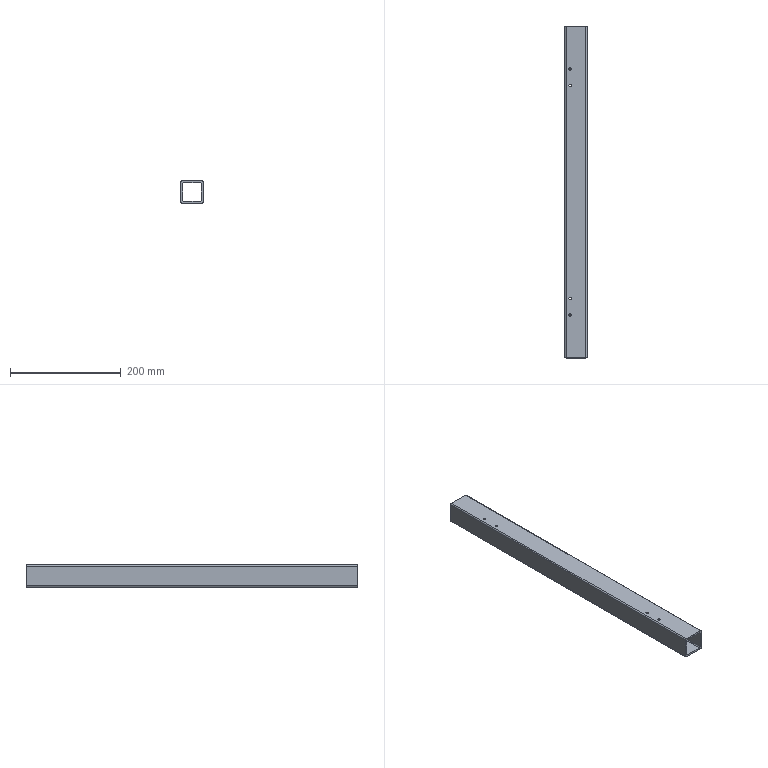Part | STEP file | SynoNew-0304-041 | 1 solid | 26 faces | box 40 x 600 x 40 mm | volume 266067 mm3 | cylinder 16 | plane 10 | commonest cylinder face diameters 4 x8 4.2 x8
STEP:
#1=CARTESIAN_POINT('',(-12.8,192.5,3.));
#2=VERTEX_POINT('',#1);
#3=CARTESIAN_POINT('',(-10.7,192.5,3.));
#4=DIRECTION('',(0.,0.,-1.));
#5=DIRECTION('',(1.,0.,0.));
#6=AXIS2_PLACEMENT_3D('',#3,#4,#5);
#7=CIRCLE('',#6,2.1);
#8=EDGE_CURVE('',#2,#2,#7,.T.);
#9=ORIENTED_EDGE('',*,*,#8,.F.);
#10=CARTESIAN_POINT('',(-12.8,192.5,0.));
#11=VERTEX_POINT('',#10);
#12=CARTESIAN_POINT('',(-12.8,192.5,-562.661));
#13=DIRECTION('',(0.,0.,-1.));
#14=VECTOR('',#13,2.1);
#15=LINE('',#12,#14);
#16=EDGE_CURVE('',#2,#11,#15,.T.);
#17=ORIENTED_EDGE('',*,*,#16,.T.);
#18=CARTESIAN_POINT('',(-10.7,192.5,0.));
#19=DIRECTION('',(0.,0.,1.));
#20=DIRECTION('',(1.,0.,0.));
#21=AXIS2_PLACEMENT_3D('',#18,#19,#20);
#22=CIRCLE('',#21,2.1);
#23=EDGE_CURVE('',#11,#11,#22,.T.);
#24=ORIENTED_EDGE('',*,*,#23,.F.);
#25=ORIENTED_EDGE('',*,*,#16,.F.);
#26=EDGE_LOOP('',(#9,#17,#24,#25));
#27=FACE_OUTER_BOUND('',#26,.T.);
#28=CARTESIAN_POINT('',(-10.7,192.5,-562.661));
#29=DIRECTION('',(0.,0.,1.));
#30=DIRECTION('',(1.,0.,0.));
#31=AXIS2_PLACEMENT_3D('',#28,#29,#30);
#32=CYLINDRICAL_SURFACE('',#31,2.1);
#33=ADVANCED_FACE('',(#27),#32,.F.);
#34=CARTESIAN_POINT('',(-8.6,192.5,40.));
#35=VERTEX_POINT('',#34);
#36=CARTESIAN_POINT('',(-12.8,192.5,40.));
#37=VERTEX_POINT('',#36);
#38=CARTESIAN_POINT('',(-10.7,192.5,40.));
#39=DIRECTION('',(0.,0.,-1.));
#40=DIRECTION('',(1.,0.,0.));
#41=AXIS2_PLACEMENT_3D('',#38,#39,#40);
#42=CIRCLE('',#41,2.1);
#43=EDGE_CURVE('',#35,#37,#42,.T.);
#44=ORIENTED_EDGE('',*,*,#43,.F.);
#45=CARTESIAN_POINT('',(-10.7,192.5,40.));
#46=DIRECTION('',(0.,0.,-1.));
#47=DIRECTION('',(1.,0.,0.));
#48=AXIS2_PLACEMENT_3D('',#45,#46,#47);
#49=CIRCLE('',#48,2.1);
#50=EDGE_CURVE('',#37,#35,#49,.T.);
#51=ORIENTED_EDGE('',*,*,#50,.F.);
#52=CARTESIAN_POINT('',(-12.8,192.5,37.));
#53=VERTEX_POINT('',#52);
#54=CARTESIAN_POINT('',(-12.8,192.5,-562.661));
#55=DIRECTION('',(0.,0.,-1.));
#56=VECTOR('',#55,2.1);
#57=LINE('',#54,#56);
#58=EDGE_CURVE('',#37,#53,#57,.T.);
#59=ORIENTED_EDGE('',*,*,#58,.T.);
#60=CARTESIAN_POINT('',(-10.7,192.5,37.));
#61=DIRECTION('',(0.,0.,1.));
#62=DIRECTION('',(1.,0.,0.));
#63=AXIS2_PLACEMENT_3D('',#60,#61,#62);
#64=CIRCLE('',#63,2.1);
#65=EDGE_CURVE('',#53,#53,#64,.T.);
#66=ORIENTED_EDGE('',*,*,#65,.F.);
#67=ORIENTED_EDGE('',*,*,#58,.F.);
#68=EDGE_LOOP('',(#44,#51,#59,#66,#67));
#69=FACE_OUTER_BOUND('',#68,.T.);
#70=CARTESIAN_POINT('',(-10.7,192.5,-562.661));
#71=DIRECTION('',(0.,0.,1.));
#72=DIRECTION('',(1.,0.,0.));
#73=AXIS2_PLACEMENT_3D('',#70,#71,#72);
#74=CYLINDRICAL_SURFACE('',#73,2.1);
#75=ADVANCED_FACE('',(#69),#74,.F.);
#76=CARTESIAN_POINT('',(-12.8,-192.5,3.));
#77=VERTEX_POINT('',#76);
#78=CARTESIAN_POINT('',(-10.7,-192.5,3.));
#79=DIRECTION('',(0.,0.,-1.));
#80=DIRECTION('',(1.,0.,0.));
#81=AXIS2_PLACEMENT_3D('',#78,#79,#80);
#82=CIRCLE('',#81,2.1);
#83=EDGE_CURVE('',#77,#77,#82,.T.);
#84=ORIENTED_EDGE('',*,*,#83,.F.);
#85=CARTESIAN_POINT('',(-12.8,-192.5,0.));
#86=VERTEX_POINT('',#85);
#87=CARTESIAN_POINT('',(-12.8,-192.5,-562.661));
#88=DIRECTION('',(0.,0.,-1.));
#89=VECTOR('',#88,2.1);
#90=LINE('',#87,#89);
#91=EDGE_CURVE('',#77,#86,#90,.T.);
#92=ORIENTED_EDGE('',*,*,#91,.T.);
#93=CARTESIAN_POINT('',(-10.7,-192.5,0.));
#94=DIRECTION('',(0.,0.,1.));
#95=DIRECTION('',(1.,0.,0.));
#96=AXIS2_PLACEMENT_3D('',#93,#94,#95);
#97=CIRCLE('',#96,2.1);
#98=EDGE_CURVE('',#86,#86,#97,.T.);
#99=ORIENTED_EDGE('',*,*,#98,.F.);
#100=ORIENTED_EDGE('',*,*,#91,.F.);
#101=EDGE_LOOP('',(#84,#92,#99,#100));
#102=FACE_OUTER_BOUND('',#101,.T.);
#103=CARTESIAN_POINT('',(-10.7,-192.5,-562.661));
#104=DIRECTION('',(0.,0.,1.));
#105=DIRECTION('',(1.,0.,0.));
#106=AXIS2_PLACEMENT_3D('',#103,#104,#105);
#107=CYLINDRICAL_SURFACE('',#106,2.1);
#108=ADVANCED_FACE('',(#102),#107,.F.);
#109=CARTESIAN_POINT('',(-8.6,-192.5,40.));
#110=VERTEX_POINT('',#109);
#111=CARTESIAN_POINT('',(-12.8,-192.5,40.));
#112=VERTEX_POINT('',#111);
#113=CARTESIAN_POINT('',(-10.7,-192.5,40.));
#114=DIRECTION('',(0.,0.,-1.));
#115=DIRECTION('',(1.,0.,0.));
#116=AXIS2_PLACEMENT_3D('',#113,#114,#115);
#117=CIRCLE('',#116,2.1);
#118=EDGE_CURVE('',#110,#112,#117,.T.);
#119=ORIENTED_EDGE('',*,*,#118,.F.);
#120=CARTESIAN_POINT('',(-10.7,-192.5,40.));
#121=DIRECTION('',(0.,0.,-1.));
#122=DIRECTION('',(1.,0.,0.));
#123=AXIS2_PLACEMENT_3D('',#120,#121,#122);
#124=CIRCLE('',#123,2.1);
#125=EDGE_CURVE('',#112,#110,#124,.T.);
#126=ORIENTED_EDGE('',*,*,#125,.F.);
#127=CARTESIAN_POINT('',(-12.8,-192.5,37.));
#128=VERTEX_POINT('',#127);
#129=CARTESIAN_POINT('',(-12.8,-192.5,-562.661));
#130=DIRECTION('',(0.,0.,-1.));
#131=VECTOR('',#130,2.1);
#132=LINE('',#129,#131);
#133=EDGE_CURVE('',#112,#128,#132,.T.);
#134=ORIENTED_EDGE('',*,*,#133,.T.);
#135=CARTESIAN_POINT('',(-10.7,-192.5,37.));
#136=DIRECTION('',(0.,0.,1.));
#137=DIRECTION('',(1.,0.,0.));
#138=AXIS2_PLACEMENT_3D('',#135,#136,#137);
#139=CIRCLE('',#138,2.1);
#140=EDGE_CURVE('',#128,#128,#139,.T.);
#141=ORIENTED_EDGE('',*,*,#140,.F.);
#142=ORIENTED_EDGE('',*,*,#133,.F.);
#143=EDGE_LOOP('',(#119,#126,#134,#141,#142));
#144=FACE_OUTER_BOUND('',#143,.T.);
#145=CARTESIAN_POINT('',(-10.7,-192.5,-562.661));
#146=DIRECTION('',(0.,0.,1.));
#147=DIRECTION('',(1.,0.,0.));
#148=AXIS2_PLACEMENT_3D('',#145,#146,#147);
#149=CYLINDRICAL_SURFACE('',#148,2.1);
#150=ADVANCED_FACE('',(#144),#149,.F.);
#151=CARTESIAN_POINT('',(-12.8,-222.5,3.));
#152=VERTEX_POINT('',#151);
#153=CARTESIAN_POINT('',(-10.7,-222.5,3.));
#154=DIRECTION('',(0.,0.,-1.));
#155=DIRECTION('',(1.,0.,0.));
#156=AXIS2_PLACEMENT_3D('',#153,#154,#155);
#157=CIRCLE('',#156,2.1);
#158=EDGE_CURVE('',#152,#152,#157,.T.);
#159=ORIENTED_EDGE('',*,*,#158,.F.);
#160=CARTESIAN_POINT('',(-12.8,-222.5,0.));
#161=VERTEX_POINT('',#160);
#162=CARTESIAN_POINT('',(-12.8,-222.5,-562.661));
#163=DIRECTION('',(0.,0.,-1.));
#164=VECTOR('',#163,2.1);
#165=LINE('',#162,#164);
#166=EDGE_CURVE('',#152,#161,#165,.T.);
#167=ORIENTED_EDGE('',*,*,#166,.T.);
#168=CARTESIAN_POINT('',(-10.7,-222.5,0.));
#169=DIRECTION('',(0.,0.,1.));
#170=DIRECTION('',(1.,0.,0.));
#171=AXIS2_PLACEMENT_3D('',#168,#169,#170);
#172=CIRCLE('',#171,2.1);
#173=EDGE_CURVE('',#161,#161,#172,.T.);
#174=ORIENTED_EDGE('',*,*,#173,.F.);
#175=ORIENTED_EDGE('',*,*,#166,.F.);
#176=EDGE_LOOP('',(#159,#167,#174,#175));
#177=FACE_OUTER_BOUND('',#176,.T.);
#178=CARTESIAN_POINT('',(-10.7,-222.5,-562.661));
#179=DIRECTION('',(0.,0.,1.));
#180=DIRECTION('',(1.,0.,0.));
#181=AXIS2_PLACEMENT_3D('',#178,#179,#180);
#182=CYLINDRICAL_SURFACE('',#181,2.1);
#183=ADVANCED_FACE('',(#177),#182,.F.);
#184=CARTESIAN_POINT('',(-8.6,-222.5,40.));
#185=VERTEX_POINT('',#184);
#186=CARTESIAN_POINT('',(-12.8,-222.5,40.));
#187=VERTEX_POINT('',#186);
#188=CARTESIAN_POINT('',(-10.7,-222.5,40.));
#189=DIRECTION('',(0.,0.,-1.));
#190=DIRECTION('',(1.,0.,0.));
#191=AXIS2_PLACEMENT_3D('',#188,#189,#190);
#192=CIRCLE('',#191,2.1);
#193=EDGE_CURVE('',#185,#187,#192,.T.);
#194=ORIENTED_EDGE('',*,*,#193,.F.);
#195=CARTESIAN_POINT('',(-10.7,-222.5,40.));
#196=DIRECTION('',(0.,0.,-1.));
#197=DIRECTION('',(1.,0.,0.));
#198=AXIS2_PLACEMENT_3D('',#195,#196,#197);
#199=CIRCLE('',#198,2.1);
#200=EDGE_CURVE('',#187,#185,#199,.T.);
#201=ORIENTED_EDGE('',*,*,#200,.F.);
#202=CARTESIAN_POINT('',(-12.8,-222.5,37.));
#203=VERTEX_POINT('',#202);
#204=CARTESIAN_POINT('',(-12.8,-222.5,-562.661));
#205=DIRECTION('',(0.,0.,-1.));
#206=VECTOR('',#205,2.1);
#207=LINE('',#204,#206);
#208=EDGE_CURVE('',#187,#203,#207,.T.);
#209=ORIENTED_EDGE('',*,*,#208,.T.);
#210=CARTESIAN_POINT('',(-10.7,-222.5,37.));
#211=DIRECTION('',(0.,0.,1.));
#212=DIRECTION('',(1.,0.,0.));
#213=AXIS2_PLACEMENT_3D('',#210,#211,#212);
#214=CIRCLE('',#213,2.1);
#215=EDGE_CURVE('',#203,#203,#214,.T.);
#216=ORIENTED_EDGE('',*,*,#215,.F.);
#217=ORIENTED_EDGE('',*,*,#208,.F.);
#218=EDGE_LOOP('',(#194,#201,#209,#216,#217));
#219=FACE_OUTER_BOUND('',#218,.T.);
#220=CARTESIAN_POINT('',(-10.7,-222.5,-562.661));
#221=DIRECTION('',(0.,0.,1.));
#222=DIRECTION('',(1.,0.,0.));
#223=AXIS2_PLACEMENT_3D('',#220,#221,#222);
#224=CYLINDRICAL_SURFACE('',#223,2.1);
#225=ADVANCED_FACE('',(#219),#224,.F.);
#226=CARTESIAN_POINT('',(-12.8,222.5,3.));
#227=VERTEX_POINT('',#226);
#228=CARTESIAN_POINT('',(-10.7,222.5,3.));
#229=DIRECTION('',(0.,0.,-1.));
#230=DIRECTION('',(1.,0.,0.));
#231=AXIS2_PLACEMENT_3D('',#228,#229,#230);
#232=CIRCLE('',#231,2.1);
#233=EDGE_CURVE('',#227,#227,#232,.T.);
#234=ORIENTED_EDGE('',*,*,#233,.F.);
#235=CARTESIAN_POINT('',(-12.8,222.5,0.));
#236=VERTEX_POINT('',#235);
#237=CARTESIAN_POINT('',(-12.8,222.5,-562.661));
#238=DIRECTION('',(0.,0.,-1.));
#239=VECTOR('',#238,2.1);
#240=LINE('',#237,#239);
#241=EDGE_CURVE('',#227,#236,#240,.T.);
#242=ORIENTED_EDGE('',*,*,#241,.T.);
#243=CARTESIAN_POINT('',(-10.7,222.5,0.));
#244=DIRECTION('',(0.,0.,1.));
#245=DIRECTION('',(1.,0.,0.));
#246=AXIS2_PLACEMENT_3D('',#243,#244,#245);
#247=CIRCLE('',#246,2.1);
#248=EDGE_CURVE('',#236,#236,#247,.T.);
#249=ORIENTED_EDGE('',*,*,#248,.F.);
#250=ORIENTED_EDGE('',*,*,#241,.F.);
#251=EDGE_LOOP('',(#234,#242,#249,#250));
#252=FACE_OUTER_BOUND('',#251,.T.);
#253=CARTESIAN_POINT('',(-10.7,222.5,-562.661));
#254=DIRECTION('',(0.,0.,1.));
#255=DIRECTION('',(1.,0.,0.));
#256=AXIS2_PLACEMENT_3D('',#253,#254,#255);
#257=CYLINDRICAL_SURFACE('',#256,2.1);
#258=ADVANCED_FACE('',(#252),#257,.F.);
#259=CARTESIAN_POINT('',(-8.6,222.5,40.));
#260=VERTEX_POINT('',#259);
#261=CARTESIAN_POINT('',(-12.8,222.5,40.));
#262=VERTEX_POINT('',#261);
#263=CARTESIAN_POINT('',(-10.7,222.5,40.));
#264=DIRECTION('',(0.,0.,-1.));
#265=DIRECTION('',(1.,0.,0.));
#266=AXIS2_PLACEMENT_3D('',#263,#264,#265);
#267=CIRCLE('',#266,2.1);
#268=EDGE_CURVE('',#260,#262,#267,.T.);
#269=ORIENTED_EDGE('',*,*,#268,.F.);
#270=CARTESIAN_POINT('',(-10.7,222.5,40.));
#271=DIRECTION('',(0.,0.,-1.));
#272=DIRECTION('',(1.,0.,0.));
#273=AXIS2_PLACEMENT_3D('',#270,#271,#272);
#274=CIRCLE('',#273,2.1);
#275=EDGE_CURVE('',#262,#260,#274,.T.);
#276=ORIENTED_EDGE('',*,*,#275,.F.);
#277=CARTESIAN_POINT('',(-12.8,222.5,37.));
#278=VERTEX_POINT('',#277);
#279=CARTESIAN_POINT('',(-12.8,222.5,-562.661));
#280=DIRECTION('',(0.,0.,-1.));
#281=VECTOR('',#280,2.1);
#282=LINE('',#279,#281);
#283=EDGE_CURVE('',#262,#278,#282,.T.);
#284=ORIENTED_EDGE('',*,*,#283,.T.);
#285=CARTESIAN_POINT('',(-10.7,222.5,37.));
#286=DIRECTION('',(0.,0.,1.));
#287=DIRECTION('',(1.,0.,0.));
#288=AXIS2_PLACEMENT_3D('',#285,#286,#287);
#289=CIRCLE('',#288,2.1);
#290=EDGE_CURVE('',#278,#278,#289,.T.);
#291=ORIENTED_EDGE('',*,*,#290,.F.);
#292=ORIENTED_EDGE('',*,*,#283,.F.);
#293=EDGE_LOOP('',(#269,#276,#284,#291,#292));
#294=FACE_OUTER_BOUND('',#293,.T.);
#295=CARTESIAN_POINT('',(-10.7,222.5,-562.661));
#296=DIRECTION('',(0.,0.,1.));
#297=DIRECTION('',(1.,0.,0.));
#298=AXIS2_PLACEMENT_3D('',#295,#296,#297);
#299=CYLINDRICAL_SURFACE('',#298,2.1);
#300=ADVANCED_FACE('',(#294),#299,.F.);
#301=CARTESIAN_POINT('',(-18.,-300.,0.));
#302=VERTEX_POINT('',#301);
#303=CARTESIAN_POINT('',(-20.,-300.,2.));
#304=VERTEX_POINT('',#303);
#305=CARTESIAN_POINT('',(-18.,-300.,2.));
#306=DIRECTION('',(0.,1.,0.));
#307=DIRECTION('',(-0.7071,0.,-0.7071));
#308=AXIS2_PLACEMENT_3D('',#305,#306,#307);
#309=CIRCLE('',#308,2.);
#310=EDGE_CURVE('',#302,#304,#309,.T.);
#311=ORIENTED_EDGE('',*,*,#310,.T.);
#312=CARTESIAN_POINT('',(-20.,300.,2.));
#313=VERTEX_POINT('',#312);
#314=CARTESIAN_POINT('',(-20.,150.,2.));
#315=DIRECTION('',(0.,1.,0.));
#316=VECTOR('',#315,10.);
#317=LINE('',#314,#316);
#318=EDGE_CURVE('',#304,#313,#317,.T.);
#319=ORIENTED_EDGE('',*,*,#318,.T.);
#320=CARTESIAN_POINT('',(-18.,300.,0.));
#321=VERTEX_POINT('',#320);
#322=CARTESIAN_POINT('',(-18.,300.,2.));
#323=DIRECTION('',(0.,-1.,0.));
#324=DIRECTION('',(-0.7071,0.,-0.7071));
#325=AXIS2_PLACEMENT_3D('',#322,#323,#324);
#326=CIRCLE('',#325,2.);
#327=EDGE_CURVE('',#313,#321,#326,.T.);
#328=ORIENTED_EDGE('',*,*,#327,.T.);
#329=CARTESIAN_POINT('',(-18.,150.,0.));
#330=DIRECTION('',(0.,-1.,0.));
#331=VECTOR('',#330,10.);
#332=LINE('',#329,#331);
#333=EDGE_CURVE('',#321,#302,#332,.T.);
#334=ORIENTED_EDGE('',*,*,#333,.T.);
#335=EDGE_LOOP('',(#311,#319,#328,#334));
#336=FACE_OUTER_BOUND('',#335,.T.);
#337=CARTESIAN_POINT('',(-18.,150.,2.));
#338=DIRECTION('',(0.,-1.,0.));
#339=DIRECTION('',(-0.7071,0.,-0.7071));
#340=AXIS2_PLACEMENT_3D('',#337,#338,#339);
#341=CYLINDRICAL_SURFACE('',#340,2.);
#342=ADVANCED_FACE('',(#336),#341,.T.);
#343=ORIENTED_EDGE('',*,*,#333,.F.);
#344=CARTESIAN_POINT('',(18.,300.,0.));
#345=VERTEX_POINT('',#344);
#346=CARTESIAN_POINT('',(20.,300.,0.));
#347=DIRECTION('',(-1.,0.,0.));
#348=VECTOR('',#347,10.);
#349=LINE('',#346,#348);
#350=EDGE_CURVE('',#345,#321,#349,.T.);
#351=ORIENTED_EDGE('',*,*,#350,.F.);
#352=CARTESIAN_POINT('',(18.,-300.,0.));
#353=VERTEX_POINT('',#352);
#354=CARTESIAN_POINT('',(18.,-150.,0.));
#355=DIRECTION('',(0.,1.,0.));
#356=VECTOR('',#355,10.);
#357=LINE('',#354,#356);
#358=EDGE_CURVE('',#353,#345,#357,.T.);
#359=ORIENTED_EDGE('',*,*,#358,.F.);
#360=CARTESIAN_POINT('',(-20.,-300.,0.));
#361=DIRECTION('',(1.,0.,0.));
#362=VECTOR('',#361,10.);
#363=LINE('',#360,#362);
#364=EDGE_CURVE('',#302,#353,#363,.T.);
#365=ORIENTED_EDGE('',*,*,#364,.F.);
#366=EDGE_LOOP('',(#343,#351,#359,#365));
#367=FACE_OUTER_BOUND('',#366,.T.);
#368=ORIENTED_EDGE('',*,*,#23,.T.);
#369=EDGE_LOOP('',(#368));
#370=FACE_BOUND('',#369,.T.);
#371=ORIENTED_EDGE('',*,*,#98,.T.);
#372=EDGE_LOOP('',(#371));
#373=FACE_BOUND('',#372,.T.);
#374=ORIENTED_EDGE('',*,*,#173,.T.);
#375=EDGE_LOOP('',(#374));
#376=FACE_BOUND('',#375,.T.);
#377=ORIENTED_EDGE('',*,*,#248,.T.);
#378=EDGE_LOOP('',(#377));
#379=FACE_BOUND('',#378,.T.);
#380=CARTESIAN_POINT('',(0.,0.,0.));
#381=DIRECTION('',(0.,0.,1.));
#382=DIRECTION('',(1.,0.,0.));
#383=AXIS2_PLACEMENT_3D('',#380,#381,#382);
#384=PLANE('',#383);
#385=ADVANCED_FACE('',(#367,#370,#373,#376,#379),#384,.F.);
#386=ORIENTED_EDGE('',*,*,#327,.F.);
#387=CARTESIAN_POINT('',(-20.,300.,38.));
#388=VERTEX_POINT('',#387);
#389=CARTESIAN_POINT('',(-20.,300.,0.));
#390=DIRECTION('',(0.,0.,1.));
#391=VECTOR('',#390,10.);
#392=LINE('',#389,#391);
#393=EDGE_CURVE('',#313,#388,#392,.T.);
#394=ORIENTED_EDGE('',*,*,#393,.T.);
#395=CARTESIAN_POINT('',(-18.,300.,40.));
#396=VERTEX_POINT('',#395);
#397=CARTESIAN_POINT('',(-18.,300.,38.));
#398=DIRECTION('',(0.,-1.,0.));
#399=DIRECTION('',(-0.7071,0.,0.7071));
#400=AXIS2_PLACEMENT_3D('',#397,#398,#399);
#401=CIRCLE('',#400,2.);
#402=EDGE_CURVE('',#396,#388,#401,.T.);
#403=ORIENTED_EDGE('',*,*,#402,.F.);
#404=CARTESIAN_POINT('',(18.,300.,40.));
#405=VERTEX_POINT('',#404);
#406=CARTESIAN_POINT('',(20.,300.,40.));
#407=DIRECTION('',(-1.,0.,0.));
#408=VECTOR('',#407,10.);
#409=LINE('',#406,#408);
#410=EDGE_CURVE('',#405,#396,#409,.T.);
#411=ORIENTED_EDGE('',*,*,#410,.F.);
#412=CARTESIAN_POINT('',(20.,300.,38.));
#413=VERTEX_POINT('',#412);
#414=CARTESIAN_POINT('',(18.,300.,38.));
#415=DIRECTION('',(0.,-1.,0.));
#416=DIRECTION('',(0.7071,0.,0.7071));
#417=AXIS2_PLACEMENT_3D('',#414,#415,#416);
#418=CIRCLE('',#417,2.);
#419=EDGE_CURVE('',#413,#405,#418,.T.);
#420=ORIENTED_EDGE('',*,*,#419,.F.);
#421=CARTESIAN_POINT('',(20.,300.,2.));
#422=VERTEX_POINT('',#421);
#423=CARTESIAN_POINT('',(20.,300.,0.));
#424=DIRECTION('',(0.,0.,1.));
#425=VECTOR('',#424,10.);
#426=LINE('',#423,#425);
#427=EDGE_CURVE('',#422,#413,#426,.T.);
#428=ORIENTED_EDGE('',*,*,#427,.F.);
#429=CARTESIAN_POINT('',(18.,300.,2.));
#430=DIRECTION('',(0.,-1.,0.));
#431=DIRECTION('',(0.7071,0.,-0.7071));
#432=AXIS2_PLACEMENT_3D('',#429,#430,#431);
#433=CIRCLE('',#432,2.);
#434=EDGE_CURVE('',#345,#422,#433,.T.);
#435=ORIENTED_EDGE('',*,*,#434,.F.);
#436=ORIENTED_EDGE('',*,*,#350,.T.);
#437=EDGE_LOOP('',(#386,#394,#403,#411,#420,#428,#435,#436));
#438=FACE_OUTER_BOUND('',#437,.T.);
#439=CARTESIAN_POINT('',(17.,300.,5.));
#440=VERTEX_POINT('',#439);
#441=CARTESIAN_POINT('',(17.,300.,35.));
#442=VERTEX_POINT('',#441);
#443=CARTESIAN_POINT('',(17.,300.,1.5));
#444=DIRECTION('',(0.,0.,1.));
#445=VECTOR('',#444,10.);
#446=LINE('',#443,#445);
#447=EDGE_CURVE('',#440,#442,#446,.T.);
#448=ORIENTED_EDGE('',*,*,#447,.T.);
#449=CARTESIAN_POINT('',(15.,300.,37.));
#450=VERTEX_POINT('',#449);
#451=CARTESIAN_POINT('',(15.,300.,35.));
#452=DIRECTION('',(0.,1.,0.));
#453=DIRECTION('',(0.7071,0.,0.7071));
#454=AXIS2_PLACEMENT_3D('',#451,#452,#453);
#455=CIRCLE('',#454,2.);
#456=EDGE_CURVE('',#450,#442,#455,.T.);
#457=ORIENTED_EDGE('',*,*,#456,.F.);
#458=CARTESIAN_POINT('',(-15.,300.,37.));
#459=VERTEX_POINT('',#458);
#460=CARTESIAN_POINT('',(18.5,300.,37.));
#461=DIRECTION('',(-1.,0.,0.));
#462=VECTOR('',#461,10.);
#463=LINE('',#460,#462);
#464=EDGE_CURVE('',#450,#459,#463,.T.);
#465=ORIENTED_EDGE('',*,*,#464,.T.);
#466=CARTESIAN_POINT('',(-17.,300.,35.));
#467=VERTEX_POINT('',#466);
#468=CARTESIAN_POINT('',(-15.,300.,35.));
#469=DIRECTION('',(0.,1.,0.));
#470=DIRECTION('',(-0.7071,0.,0.7071));
#471=AXIS2_PLACEMENT_3D('',#468,#469,#470);
#472=CIRCLE('',#471,2.);
#473=EDGE_CURVE('',#467,#459,#472,.T.);
#474=ORIENTED_EDGE('',*,*,#473,.F.);
#475=CARTESIAN_POINT('',(-17.,300.,5.));
#476=VERTEX_POINT('',#475);
#477=CARTESIAN_POINT('',(-17.,300.,18.5));
#478=DIRECTION('',(0.,0.,-1.));
#479=VECTOR('',#478,10.);
#480=LINE('',#477,#479);
#481=EDGE_CURVE('',#467,#476,#480,.T.);
#482=ORIENTED_EDGE('',*,*,#481,.T.);
#483=CARTESIAN_POINT('',(-15.,300.,3.));
#484=VERTEX_POINT('',#483);
#485=CARTESIAN_POINT('',(-15.,300.,5.));
#486=DIRECTION('',(0.,1.,0.));
#487=DIRECTION('',(-0.7071,0.,-0.7071));
#488=AXIS2_PLACEMENT_3D('',#485,#486,#487);
#489=CIRCLE('',#488,2.);
#490=EDGE_CURVE('',#484,#476,#489,.T.);
#491=ORIENTED_EDGE('',*,*,#490,.F.);
#492=CARTESIAN_POINT('',(15.,300.,3.));
#493=VERTEX_POINT('',#492);
#494=CARTESIAN_POINT('',(1.5,300.,3.));
#495=DIRECTION('',(1.,0.,0.));
#496=VECTOR('',#495,10.);
#497=LINE('',#494,#496);
#498=EDGE_CURVE('',#484,#493,#497,.T.);
#499=ORIENTED_EDGE('',*,*,#498,.T.);
#500=CARTESIAN_POINT('',(15.,300.,5.));
#501=DIRECTION('',(0.,1.,0.));
#502=DIRECTION('',(0.7071,0.,-0.7071));
#503=AXIS2_PLACEMENT_3D('',#500,#501,#502);
#504=CIRCLE('',#503,2.);
#505=EDGE_CURVE('',#440,#493,#504,.T.);
#506=ORIENTED_EDGE('',*,*,#505,.F.);
#507=EDGE_LOOP('',(#448,#457,#465,#474,#482,#491,#499,#506));
#508=FACE_BOUND('',#507,.T.);
#509=CARTESIAN_POINT('',(20.,300.,0.));
#510=DIRECTION('',(0.,1.,0.));
#511=DIRECTION('',(-1.,0.,0.));
#512=AXIS2_PLACEMENT_3D('',#509,#510,#511);
#513=PLANE('',#512);
#514=ADVANCED_FACE('',(#438,#508),#513,.T.);
#515=ORIENTED_EDGE('',*,*,#490,.T.);
#516=CARTESIAN_POINT('',(-17.,-300.,5.));
#517=VERTEX_POINT('',#516);
#518=CARTESIAN_POINT('',(-17.,300.,5.));
#519=DIRECTION('',(0.,-1.,0.));
#520=VECTOR('',#519,10.);
#521=LINE('',#518,#520);
#522=EDGE_CURVE('',#476,#517,#521,.T.);
#523=ORIENTED_EDGE('',*,*,#522,.T.);
#524=CARTESIAN_POINT('',(-15.,-300.,3.));
#525=VERTEX_POINT('',#524);
#526=CARTESIAN_POINT('',(-15.,-300.,5.));
#527=DIRECTION('',(0.,-1.,0.));
#528=DIRECTION('',(-0.7071,0.,-0.7071));
#529=AXIS2_PLACEMENT_3D('',#526,#527,#528);
#530=CIRCLE('',#529,2.);
#531=EDGE_CURVE('',#517,#525,#530,.T.);
#532=ORIENTED_EDGE('',*,*,#531,.T.);
#533=CARTESIAN_POINT('',(-15.,300.,3.));
#534=DIRECTION('',(0.,1.,0.));
#535=VECTOR('',#534,10.);
#536=LINE('',#533,#535);
#537=EDGE_CURVE('',#525,#484,#536,.T.);
#538=ORIENTED_EDGE('',*,*,#537,.T.);
#539=EDGE_LOOP('',(#515,#523,#532,#538));
#540=FACE_OUTER_BOUND('',#539,.T.);
#541=CARTESIAN_POINT('',(-15.,300.,5.));
#542=DIRECTION('',(0.,-1.,0.));
#543=DIRECTION('',(-0.7071,0.,-0.7071));
#544=AXIS2_PLACEMENT_3D('',#541,#542,#543);
#545=CYLINDRICAL_SURFACE('',#544,2.);
#546=ADVANCED_FACE('',(#540),#545,.F.);
#547=ORIENTED_EDGE('',*,*,#522,.F.);
#548=ORIENTED_EDGE('',*,*,#481,.F.);
#549=CARTESIAN_POINT('',(-17.,-300.,35.));
#550=VERTEX_POINT('',#549);
#551=CARTESIAN_POINT('',(-17.,300.,35.));
#552=DIRECTION('',(0.,1.,0.));
#553=VECTOR('',#552,10.);
#554=LINE('',#551,#553);
#555=EDGE_CURVE('',#550,#467,#554,.T.);
#556=ORIENTED_EDGE('',*,*,#555,.F.);
#557=CARTESIAN_POINT('',(-17.,-300.,18.5));
#558=DIRECTION('',(0.,0.,1.));
#559=VECTOR('',#558,10.);
#560=LINE('',#557,#559);
#561=EDGE_CURVE('',#517,#550,#560,.T.);
#562=ORIENTED_EDGE('',*,*,#561,.F.);
#563=EDGE_LOOP('',(#547,#548,#556,#562));
#564=FACE_OUTER_BOUND('',#563,.T.);
#565=CARTESIAN_POINT('',(-17.,300.,37.));
#566=DIRECTION('',(-1.,0.,0.));
#567=DIRECTION('',(0.,0.,-1.));
#568=AXIS2_PLACEMENT_3D('',#565,#566,#567);
#569=PLANE('',#568);
#570=ADVANCED_FACE('',(#564),#569,.F.);
#571=ORIENTED_EDGE('',*,*,#473,.T.);
#572=CARTESIAN_POINT('',(-15.,-300.,37.));
#573=VERTEX_POINT('',#572);
#574=CARTESIAN_POINT('',(-15.,300.,37.));
#575=DIRECTION('',(0.,-1.,0.));
#576=VECTOR('',#575,10.);
#577=LINE('',#574,#576);
#578=EDGE_CURVE('',#459,#573,#577,.T.);
#579=ORIENTED_EDGE('',*,*,#578,.T.);
#580=CARTESIAN_POINT('',(-15.,-300.,35.));
#581=DIRECTION('',(0.,-1.,0.));
#582=DIRECTION('',(-0.7071,0.,0.7071));
#583=AXIS2_PLACEMENT_3D('',#580,#581,#582);
#584=CIRCLE('',#583,2.);
#585=EDGE_CURVE('',#573,#550,#584,.T.);
#586=ORIENTED_EDGE('',*,*,#585,.T.);
#587=ORIENTED_EDGE('',*,*,#555,.T.);
#588=EDGE_LOOP('',(#571,#579,#586,#587));
#589=FACE_OUTER_BOUND('',#588,.T.);
#590=CARTESIAN_POINT('',(-15.,300.,35.));
#591=DIRECTION('',(0.,-1.,0.));
#592=DIRECTION('',(-0.7071,0.,0.7071));
#593=AXIS2_PLACEMENT_3D('',#590,#591,#592);
#594=CYLINDRICAL_SURFACE('',#593,2.);
#595=ADVANCED_FACE('',(#589),#594,.F.);
#596=ORIENTED_EDGE('',*,*,#578,.F.);
#597=ORIENTED_EDGE('',*,*,#464,.F.);
#598=CARTESIAN_POINT('',(15.,-300.,37.));
#599=VERTEX_POINT('',#598);
#600=CARTESIAN_POINT('',(15.,300.,37.));
#601=DIRECTION('',(0.,1.,0.));
#602=VECTOR('',#601,10.);
#603=LINE('',#600,#602);
#604=EDGE_CURVE('',#599,#450,#603,.T.);
#605=ORIENTED_EDGE('',*,*,#604,.F.);
#606=CARTESIAN_POINT('',(-1.5,-300.,37.));
#607=DIRECTION('',(1.,0.,0.));
#608=VECTOR('',#607,10.);
#609=LINE('',#606,#608);
#610=EDGE_CURVE('',#573,#599,#609,.T.);
#611=ORIENTED_EDGE('',*,*,#610,.F.);
#612=EDGE_LOOP('',(#596,#597,#605,#611));
#613=FACE_OUTER_BOUND('',#612,.T.);
#614=ORIENTED_EDGE('',*,*,#65,.T.);
#615=EDGE_LOOP('',(#614));
#616=FACE_BOUND('',#615,.T.);
#617=ORIENTED_EDGE('',*,*,#140,.T.);
#618=EDGE_LOOP('',(#617));
#619=FACE_BOUND('',#618,.T.);
#620=ORIENTED_EDGE('',*,*,#215,.T.);
#621=EDGE_LOOP('',(#620));
#622=FACE_BOUND('',#621,.T.);
#623=ORIENTED_EDGE('',*,*,#290,.T.);
#624=EDGE_LOOP('',(#623));
#625=FACE_BOUND('',#624,.T.);
#626=CARTESIAN_POINT('',(17.,300.,37.));
#627=DIRECTION('',(0.,0.,1.));
#628=DIRECTION('',(-1.,0.,0.));
#629=AXIS2_PLACEMENT_3D('',#626,#627,#628);
#630=PLANE('',#629);
#631=ADVANCED_FACE('',(#613,#616,#619,#622,#625),#630,.F.);
#632=CARTESIAN_POINT('',(-20.,-300.,38.));
#633=VERTEX_POINT('',#632);
#634=CARTESIAN_POINT('',(-18.,-300.,40.));
#635=VERTEX_POINT('',#634);
#636=CARTESIAN_POINT('',(-18.,-300.,38.));
#637=DIRECTION('',(0.,1.,0.));
#638=DIRECTION('',(-0.7071,0.,0.7071));
#639=AXIS2_PLACEMENT_3D('',#636,#637,#638);
#640=CIRCLE('',#639,2.);
#641=EDGE_CURVE('',#633,#635,#640,.T.);
#642=ORIENTED_EDGE('',*,*,#641,.T.);
#643=CARTESIAN_POINT('',(-18.,150.,40.));
#644=DIRECTION('',(0.,1.,0.));
#645=VECTOR('',#644,10.);
#646=LINE('',#643,#645);
#647=EDGE_CURVE('',#635,#396,#646,.T.);
#648=ORIENTED_EDGE('',*,*,#647,.T.);
#649=ORIENTED_EDGE('',*,*,#402,.T.);
#650=CARTESIAN_POINT('',(-20.,150.,38.));
#651=DIRECTION('',(0.,-1.,0.));
#652=VECTOR('',#651,10.);
#653=LINE('',#650,#652);
#654=EDGE_CURVE('',#388,#633,#653,.T.);
#655=ORIENTED_EDGE('',*,*,#654,.T.);
#656=EDGE_LOOP('',(#642,#648,#649,#655));
#657=FACE_OUTER_BOUND('',#656,.T.);
#658=CARTESIAN_POINT('',(-18.,150.,38.));
#659=DIRECTION('',(0.,-1.,0.));
#660=DIRECTION('',(-0.7071,0.,0.7071));
#661=AXIS2_PLACEMENT_3D('',#658,#659,#660);
#662=CYLINDRICAL_SURFACE('',#661,2.);
#663=ADVANCED_FACE('',(#657),#662,.T.);
#664=ORIENTED_EDGE('',*,*,#647,.F.);
#665=CARTESIAN_POINT('',(18.,-300.,40.));
#666=VERTEX_POINT('',#665);
#667=CARTESIAN_POINT('',(-20.,-300.,40.));
#668=DIRECTION('',(1.,0.,0.));
#669=VECTOR('',#668,10.);
#670=LINE('',#667,#669);
#671=EDGE_CURVE('',#635,#666,#670,.T.);
#672=ORIENTED_EDGE('',*,*,#671,.T.);
#673=CARTESIAN_POINT('',(18.,-150.,40.));
#674=DIRECTION('',(0.,-1.,0.));
#675=VECTOR('',#674,10.);
#676=LINE('',#673,#675);
#677=EDGE_CURVE('',#405,#666,#676,.T.);
#678=ORIENTED_EDGE('',*,*,#677,.F.);
#679=ORIENTED_EDGE('',*,*,#410,.T.);
#680=EDGE_LOOP('',(#664,#672,#678,#679));
#681=FACE_OUTER_BOUND('',#680,.T.);
#682=ORIENTED_EDGE('',*,*,#43,.T.);
#683=ORIENTED_EDGE('',*,*,#50,.T.);
#684=EDGE_LOOP('',(#682,#683));
#685=FACE_BOUND('',#684,.T.);
#686=ORIENTED_EDGE('',*,*,#118,.T.);
#687=ORIENTED_EDGE('',*,*,#125,.T.);
#688=EDGE_LOOP('',(#686,#687));
#689=FACE_BOUND('',#688,.T.);
#690=ORIENTED_EDGE('',*,*,#193,.T.);
#691=ORIENTED_EDGE('',*,*,#200,.T.);
#692=EDGE_LOOP('',(#690,#691));
#693=FACE_BOUND('',#692,.T.);
#694=ORIENTED_EDGE('',*,*,#268,.T.);
#695=ORIENTED_EDGE('',*,*,#275,.T.);
#696=EDGE_LOOP('',(#694,#695));
#697=FACE_BOUND('',#696,.T.);
#698=CARTESIAN_POINT('',(0.,0.,40.));
#699=DIRECTION('',(0.,0.,1.));
#700=DIRECTION('',(1.,0.,0.));
#701=AXIS2_PLACEMENT_3D('',#698,#699,#700);
#702=PLANE('',#701);
#703=ADVANCED_FACE('',(#681,#685,#689,#693,#697),#702,.T.);
#704=ORIENTED_EDGE('',*,*,#310,.F.);
#705=ORIENTED_EDGE('',*,*,#364,.T.);
#706=CARTESIAN_POINT('',(20.,-300.,2.));
#707=VERTEX_POINT('',#706);
#708=CARTESIAN_POINT('',(18.,-300.,2.));
#709=DIRECTION('',(0.,1.,0.));
#710=DIRECTION('',(0.7071,0.,-0.7071));
#711=AXIS2_PLACEMENT_3D('',#708,#709,#710);
#712=CIRCLE('',#711,2.);
#713=EDGE_CURVE('',#707,#353,#712,.T.);
#714=ORIENTED_EDGE('',*,*,#713,.F.);
#715=CARTESIAN_POINT('',(20.,-300.,38.));
#716=VERTEX_POINT('',#715);
#717=CARTESIAN_POINT('',(20.,-300.,0.));
#718=DIRECTION('',(0.,0.,1.));
#719=VECTOR('',#718,10.);
#720=LINE('',#717,#719);
#721=EDGE_CURVE('',#707,#716,#720,.T.);
#722=ORIENTED_EDGE('',*,*,#721,.T.);
#723=CARTESIAN_POINT('',(18.,-300.,38.));
#724=DIRECTION('',(0.,1.,0.));
#725=DIRECTION('',(0.7071,0.,0.7071));
#726=AXIS2_PLACEMENT_3D('',#723,#724,#725);
#727=CIRCLE('',#726,2.);
#728=EDGE_CURVE('',#666,#716,#727,.T.);
#729=ORIENTED_EDGE('',*,*,#728,.F.);
#730=ORIENTED_EDGE('',*,*,#671,.F.);
#731=ORIENTED_EDGE('',*,*,#641,.F.);
#732=CARTESIAN_POINT('',(-20.,-300.,0.));
#733=DIRECTION('',(0.,0.,1.));
#734=VECTOR('',#733,10.);
#735=LINE('',#732,#734);
#736=EDGE_CURVE('',#304,#633,#735,.T.);
#737=ORIENTED_EDGE('',*,*,#736,.F.);
#738=EDGE_LOOP('',(#704,#705,#714,#722,#729,#730,#731,#737));
#739=FACE_OUTER_BOUND('',#738,.T.);
#740=CARTESIAN_POINT('',(17.,-300.,35.));
#741=VERTEX_POINT('',#740);
#742=CARTESIAN_POINT('',(17.,-300.,5.));
#743=VERTEX_POINT('',#742);
#744=CARTESIAN_POINT('',(17.,-300.,1.5));
#745=DIRECTION('',(0.,0.,-1.));
#746=VECTOR('',#745,10.);
#747=LINE('',#744,#746);
#748=EDGE_CURVE('',#741,#743,#747,.T.);
#749=ORIENTED_EDGE('',*,*,#748,.T.);
#750=CARTESIAN_POINT('',(15.,-300.,3.));
#751=VERTEX_POINT('',#750);
#752=CARTESIAN_POINT('',(15.,-300.,5.));
#753=DIRECTION('',(0.,-1.,0.));
#754=DIRECTION('',(0.7071,0.,-0.7071));
#755=AXIS2_PLACEMENT_3D('',#752,#753,#754);
#756=CIRCLE('',#755,2.);
#757=EDGE_CURVE('',#751,#743,#756,.T.);
#758=ORIENTED_EDGE('',*,*,#757,.F.);
#759=CARTESIAN_POINT('',(-18.5,-300.,3.));
#760=DIRECTION('',(-1.,0.,0.));
#761=VECTOR('',#760,10.);
#762=LINE('',#759,#761);
#763=EDGE_CURVE('',#751,#525,#762,.T.);
#764=ORIENTED_EDGE('',*,*,#763,.T.);
#765=ORIENTED_EDGE('',*,*,#531,.F.);
#766=ORIENTED_EDGE('',*,*,#561,.T.);
#767=ORIENTED_EDGE('',*,*,#585,.F.);
#768=ORIENTED_EDGE('',*,*,#610,.T.);
#769=CARTESIAN_POINT('',(15.,-300.,35.));
#770=DIRECTION('',(0.,-1.,0.));
#771=DIRECTION('',(0.7071,0.,0.7071));
#772=AXIS2_PLACEMENT_3D('',#769,#770,#771);
#773=CIRCLE('',#772,2.);
#774=EDGE_CURVE('',#741,#599,#773,.T.);
#775=ORIENTED_EDGE('',*,*,#774,.F.);
#776=EDGE_LOOP('',(#749,#758,#764,#765,#766,#767,#768,#775));
#777=FACE_BOUND('',#776,.T.);
#778=CARTESIAN_POINT('',(-20.,-300.,0.));
#779=DIRECTION('',(0.,-1.,0.));
#780=DIRECTION('',(1.,0.,0.));
#781=AXIS2_PLACEMENT_3D('',#778,#779,#780);
#782=PLANE('',#781);
#783=ADVANCED_FACE('',(#739,#777),#782,.T.);
#784=ORIENTED_EDGE('',*,*,#456,.T.);
#785=CARTESIAN_POINT('',(17.,300.,35.));
#786=DIRECTION('',(0.,-1.,0.));
#787=VECTOR('',#786,10.);
#788=LINE('',#785,#787);
#789=EDGE_CURVE('',#442,#741,#788,.T.);
#790=ORIENTED_EDGE('',*,*,#789,.T.);
#791=ORIENTED_EDGE('',*,*,#774,.T.);
#792=ORIENTED_EDGE('',*,*,#604,.T.);
#793=EDGE_LOOP('',(#784,#790,#791,#792));
#794=FACE_OUTER_BOUND('',#793,.T.);
#795=CARTESIAN_POINT('',(15.,300.,35.));
#796=DIRECTION('',(0.,-1.,0.));
#797=DIRECTION('',(0.7071,0.,0.7071));
#798=AXIS2_PLACEMENT_3D('',#795,#796,#797);
#799=CYLINDRICAL_SURFACE('',#798,2.);
#800=ADVANCED_FACE('',(#794),#799,.F.);
#801=ORIENTED_EDGE('',*,*,#789,.F.);
#802=ORIENTED_EDGE('',*,*,#447,.F.);
#803=CARTESIAN_POINT('',(17.,300.,5.));
#804=DIRECTION('',(0.,1.,0.));
#805=VECTOR('',#804,10.);
#806=LINE('',#803,#805);
#807=EDGE_CURVE('',#743,#440,#806,.T.);
#808=ORIENTED_EDGE('',*,*,#807,.F.);
#809=ORIENTED_EDGE('',*,*,#748,.F.);
#810=EDGE_LOOP('',(#801,#802,#808,#809));
#811=FACE_OUTER_BOUND('',#810,.T.);
#812=CARTESIAN_POINT('',(17.,300.,3.));
#813=DIRECTION('',(1.,0.,0.));
#814=DIRECTION('',(0.,0.,1.));
#815=AXIS2_PLACEMENT_3D('',#812,#813,#814);
#816=PLANE('',#815);
#817=ADVANCED_FACE('',(#811),#816,.F.);
#818=ORIENTED_EDGE('',*,*,#419,.T.);
#819=ORIENTED_EDGE('',*,*,#677,.T.);
#820=ORIENTED_EDGE('',*,*,#728,.T.);
#821=CARTESIAN_POINT('',(20.,-150.,38.));
#822=DIRECTION('',(0.,1.,0.));
#823=VECTOR('',#822,10.);
#824=LINE('',#821,#823);
#825=EDGE_CURVE('',#716,#413,#824,.T.);
#826=ORIENTED_EDGE('',*,*,#825,.T.);
#827=EDGE_LOOP('',(#818,#819,#820,#826));
#828=FACE_OUTER_BOUND('',#827,.T.);
#829=CARTESIAN_POINT('',(18.,-150.,38.));
#830=DIRECTION('',(0.,1.,0.));
#831=DIRECTION('',(0.7071,0.,0.7071));
#832=AXIS2_PLACEMENT_3D('',#829,#830,#831);
#833=CYLINDRICAL_SURFACE('',#832,2.);
#834=ADVANCED_FACE('',(#828),#833,.T.);
#835=ORIENTED_EDGE('',*,*,#825,.F.);
#836=ORIENTED_EDGE('',*,*,#721,.F.);
#837=CARTESIAN_POINT('',(20.,-150.,2.));
#838=DIRECTION('',(0.,-1.,0.));
#839=VECTOR('',#838,10.);
#840=LINE('',#837,#839);
#841=EDGE_CURVE('',#422,#707,#840,.T.);
#842=ORIENTED_EDGE('',*,*,#841,.F.);
#843=ORIENTED_EDGE('',*,*,#427,.T.);
#844=EDGE_LOOP('',(#835,#836,#842,#843));
#845=FACE_OUTER_BOUND('',#844,.T.);
#846=CARTESIAN_POINT('',(20.,-300.,0.));
#847=DIRECTION('',(1.,0.,0.));
#848=DIRECTION('',(0.,1.,0.));
#849=AXIS2_PLACEMENT_3D('',#846,#847,#848);
#850=PLANE('',#849);
#851=ADVANCED_FACE('',(#845),#850,.T.);
#852=ORIENTED_EDGE('',*,*,#434,.T.);
#853=ORIENTED_EDGE('',*,*,#841,.T.);
#854=ORIENTED_EDGE('',*,*,#713,.T.);
#855=ORIENTED_EDGE('',*,*,#358,.T.);
#856=EDGE_LOOP('',(#852,#853,#854,#855));
#857=FACE_OUTER_BOUND('',#856,.T.);
#858=CARTESIAN_POINT('',(18.,-150.,2.));
#859=DIRECTION('',(0.,1.,0.));
#860=DIRECTION('',(0.7071,0.,-0.7071));
#861=AXIS2_PLACEMENT_3D('',#858,#859,#860);
#862=CYLINDRICAL_SURFACE('',#861,2.);
#863=ADVANCED_FACE('',(#857),#862,.T.);
#864=ORIENTED_EDGE('',*,*,#505,.T.);
#865=CARTESIAN_POINT('',(15.,300.,3.));
#866=DIRECTION('',(0.,-1.,0.));
#867=VECTOR('',#866,10.);
#868=LINE('',#865,#867);
#869=EDGE_CURVE('',#493,#751,#868,.T.);
#870=ORIENTED_EDGE('',*,*,#869,.T.);
#871=ORIENTED_EDGE('',*,*,#757,.T.);
#872=ORIENTED_EDGE('',*,*,#807,.T.);
#873=EDGE_LOOP('',(#864,#870,#871,#872));
#874=FACE_OUTER_BOUND('',#873,.T.);
#875=CARTESIAN_POINT('',(15.,300.,5.));
#876=DIRECTION('',(0.,-1.,0.));
#877=DIRECTION('',(0.7071,0.,-0.7071));
#878=AXIS2_PLACEMENT_3D('',#875,#876,#877);
#879=CYLINDRICAL_SURFACE('',#878,2.);
#880=ADVANCED_FACE('',(#874),#879,.F.);
#881=ORIENTED_EDGE('',*,*,#537,.F.);
#882=ORIENTED_EDGE('',*,*,#763,.F.);
#883=ORIENTED_EDGE('',*,*,#869,.F.);
#884=ORIENTED_EDGE('',*,*,#498,.F.);
#885=EDGE_LOOP('',(#881,#882,#883,#884));
#886=FACE_OUTER_BOUND('',#885,.T.);
#887=ORIENTED_EDGE('',*,*,#8,.T.);
#888=EDGE_LOOP('',(#887));
#889=FACE_BOUND('',#888,.T.);
#890=ORIENTED_EDGE('',*,*,#83,.T.);
#891=EDGE_LOOP('',(#890));
#892=FACE_BOUND('',#891,.T.);
#893=ORIENTED_EDGE('',*,*,#158,.T.);
#894=EDGE_LOOP('',(#893));
#895=FACE_BOUND('',#894,.T.);
#896=ORIENTED_EDGE('',*,*,#233,.T.);
#897=EDGE_LOOP('',(#896));
#898=FACE_BOUND('',#897,.T.);
#899=CARTESIAN_POINT('',(-17.,300.,3.));
#900=DIRECTION('',(0.,0.,-1.));
#901=DIRECTION('',(1.,0.,0.));
#902=AXIS2_PLACEMENT_3D('',#899,#900,#901);
#903=PLANE('',#902);
#904=ADVANCED_FACE('',(#886,#889,#892,#895,#898),#903,.F.);
#905=ORIENTED_EDGE('',*,*,#318,.F.);
#906=ORIENTED_EDGE('',*,*,#736,.T.);
#907=ORIENTED_EDGE('',*,*,#654,.F.);
#908=ORIENTED_EDGE('',*,*,#393,.F.);
#909=EDGE_LOOP('',(#905,#906,#907,#908));
#910=FACE_OUTER_BOUND('',#909,.T.);
#911=CARTESIAN_POINT('',(-20.,300.,0.));
#912=DIRECTION('',(-1.,0.,0.));
#913=DIRECTION('',(0.,-1.,0.));
#914=AXIS2_PLACEMENT_3D('',#911,#912,#913);
#915=PLANE('',#914);
#916=ADVANCED_FACE('',(#910),#915,.T.);
#917=CLOSED_SHELL('',(#33,#75,#108,#150,#183,#225,#258,#300,#342,#385,#514,#546,#570,#595,#631,#663,#703,#783,#800,#817,#834,#851,#863,#880,#904,#916));
#918=MANIFOLD_SOLID_BREP('',#917);
#919=(LENGTH_UNIT()NAMED_UNIT(*)SI_UNIT(.MILLI.,.METRE.));
#920=UNCERTAINTY_MEASURE_WITH_UNIT(LENGTH_MEASURE(0.01),#919,'','');
#921=(NAMED_UNIT(*)PLANE_ANGLE_UNIT()SI_UNIT($,.RADIAN.));
#922=(NAMED_UNIT(*)SI_UNIT($,.STERADIAN.)SOLID_ANGLE_UNIT());
#923=(GEOMETRIC_REPRESENTATION_CONTEXT(3)GLOBAL_UNCERTAINTY_ASSIGNED_CONTEXT((#920))GLOBAL_UNIT_ASSIGNED_CONTEXT((#919,#921,#922))REPRESENTATION_CONTEXT('',''));
#924=ADVANCED_BREP_SHAPE_REPRESENTATION('',(#918),#923);